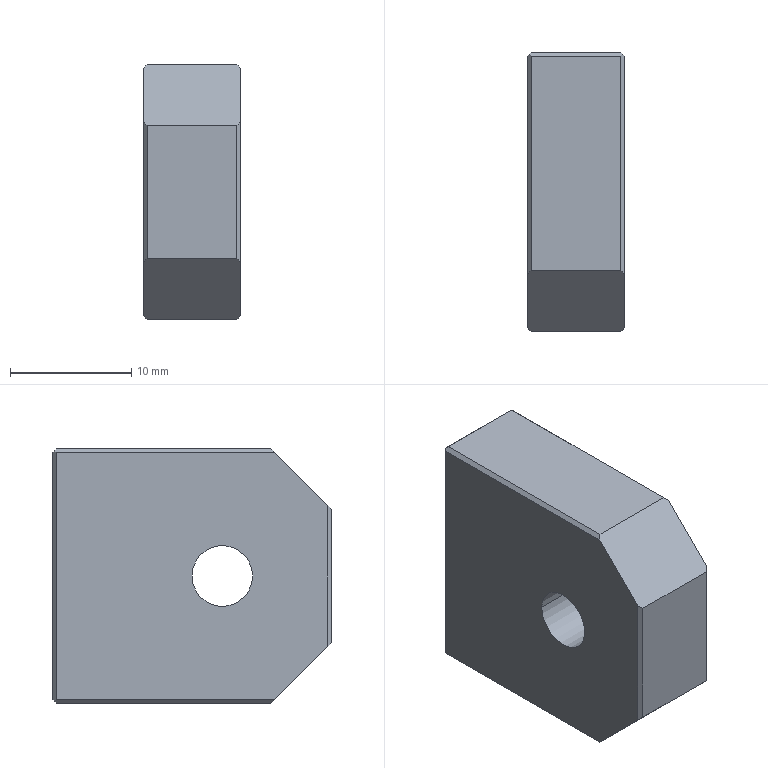Part | NX | 1 solid | 38 faces | box 8 x 23 x 21 mm | volume 3278 mm3 | plane 18 | cylinder 10 | cone 10 | commonest cylinder face diameters 3.3 x8 5 x2
STEP:
#1=CARTESIAN_POINT('',(-167.3,281.,-24.329));
#2=VERTEX_POINT('',#1);
#3=CARTESIAN_POINT('',(-174.7,281.,-24.329));
#4=VERTEX_POINT('',#3);
#5=CARTESIAN_POINT('',(-171.,281.,-24.329));
#6=DIRECTION('',(-1.,0.,0.));
#7=VECTOR('',#6,1000.);
#8=LINE('',#5,#7);
#9=EDGE_CURVE('',#2,#4,#8,.T.);
#10=ORIENTED_EDGE('',*,*,#9,.F.);
#11=CARTESIAN_POINT('',(-167.3,281.,-44.729));
#12=VERTEX_POINT('',#11);
#13=CARTESIAN_POINT('',(-167.3,281.,-34.529));
#14=DIRECTION('',(0.,0.,1.));
#15=VECTOR('',#14,1000.);
#16=LINE('',#13,#15);
#17=EDGE_CURVE('',#12,#2,#16,.T.);
#18=ORIENTED_EDGE('',*,*,#17,.F.);
#19=CARTESIAN_POINT('',(-174.7,281.,-44.729));
#20=VERTEX_POINT('',#19);
#21=CARTESIAN_POINT('',(-171.,281.,-44.729));
#22=DIRECTION('',(1.,0.,0.));
#23=VECTOR('',#22,1000.);
#24=LINE('',#21,#23);
#25=EDGE_CURVE('',#20,#12,#24,.T.);
#26=ORIENTED_EDGE('',*,*,#25,.F.);
#27=CARTESIAN_POINT('',(-174.7,281.,-34.529));
#28=DIRECTION('',(0.,0.,1.));
#29=VECTOR('',#28,1000.);
#30=LINE('',#27,#29);
#31=EDGE_CURVE('',#20,#4,#30,.T.);
#32=ORIENTED_EDGE('',*,*,#31,.T.);
#33=EDGE_LOOP('',(#10,#18,#26,#32));
#34=FACE_BOUND('',#33,.T.);
#35=CARTESIAN_POINT('',(-171.,281.,-37.464));
#36=VERTEX_POINT('',#35);
#37=CARTESIAN_POINT('',(-171.,281.,-42.094));
#38=VERTEX_POINT('',#37);
#39=CARTESIAN_POINT('',(-171.,281.,-39.779));
#40=DIRECTION('',(0.,1.,0.));
#41=DIRECTION('',(0.,0.,-1.));
#42=AXIS2_PLACEMENT_3D('',#39,#40,#41);
#43=CIRCLE('',#42,2.315);
#44=EDGE_CURVE('',#36,#38,#43,.T.);
#45=ORIENTED_EDGE('',*,*,#44,.F.);
#46=CARTESIAN_POINT('',(-171.,281.,-39.779));
#47=DIRECTION('',(0.,1.,0.));
#48=DIRECTION('',(0.,0.,-1.));
#49=AXIS2_PLACEMENT_3D('',#46,#47,#48);
#50=CIRCLE('',#49,2.315);
#51=EDGE_CURVE('',#38,#36,#50,.T.);
#52=ORIENTED_EDGE('',*,*,#51,.F.);
#53=EDGE_LOOP('',(#45,#52));
#54=FACE_BOUND('',#53,.T.);
#55=CARTESIAN_POINT('',(-171.,281.,-27.328));
#56=VERTEX_POINT('',#55);
#57=CARTESIAN_POINT('',(-171.,281.,-31.958));
#58=VERTEX_POINT('',#57);
#59=CARTESIAN_POINT('',(-171.,281.,-29.643));
#60=DIRECTION('',(0.,1.,0.));
#61=DIRECTION('',(0.,0.,-1.));
#62=AXIS2_PLACEMENT_3D('',#59,#60,#61);
#63=CIRCLE('',#62,2.315);
#64=EDGE_CURVE('',#56,#58,#63,.T.);
#65=ORIENTED_EDGE('',*,*,#64,.F.);
#66=CARTESIAN_POINT('',(-171.,281.,-29.643));
#67=DIRECTION('',(0.,1.,0.));
#68=DIRECTION('',(0.,0.,-1.));
#69=AXIS2_PLACEMENT_3D('',#66,#67,#68);
#70=CIRCLE('',#69,2.315);
#71=EDGE_CURVE('',#58,#56,#70,.T.);
#72=ORIENTED_EDGE('',*,*,#71,.F.);
#73=EDGE_LOOP('',(#65,#72));
#74=FACE_BOUND('',#73,.T.);
#75=CARTESIAN_POINT('',(-167.,281.,-45.029));
#76=DIRECTION('',(0.,1.,0.));
#77=DIRECTION('',(1.,0.,0.));
#78=AXIS2_PLACEMENT_3D('',#75,#76,#77);
#79=PLANE('',#78);
#80=ADVANCED_FACE('',(#34,#54,#74),#79,.T.);
#81=CARTESIAN_POINT('',(-167.3,263.,-45.029));
#82=VERTEX_POINT('',#81);
#83=CARTESIAN_POINT('',(-174.7,263.,-45.029));
#84=VERTEX_POINT('',#83);
#85=CARTESIAN_POINT('',(-171.,263.,-45.029));
#86=DIRECTION('',(-1.,0.,0.));
#87=VECTOR('',#86,1000.);
#88=LINE('',#85,#87);
#89=EDGE_CURVE('',#82,#84,#88,.T.);
#90=ORIENTED_EDGE('',*,*,#89,.T.);
#91=CARTESIAN_POINT('',(-174.7,280.7,-45.029));
#92=VERTEX_POINT('',#91);
#93=CARTESIAN_POINT('',(-174.7,272.,-45.029));
#94=DIRECTION('',(0.,1.,0.));
#95=VECTOR('',#94,1000.);
#96=LINE('',#93,#95);
#97=EDGE_CURVE('',#84,#92,#96,.T.);
#98=ORIENTED_EDGE('',*,*,#97,.T.);
#99=CARTESIAN_POINT('',(-167.3,280.7,-45.029));
#100=VERTEX_POINT('',#99);
#101=CARTESIAN_POINT('',(-171.,280.7,-45.029));
#102=DIRECTION('',(1.,0.,0.));
#103=VECTOR('',#102,1000.);
#104=LINE('',#101,#103);
#105=EDGE_CURVE('',#92,#100,#104,.T.);
#106=ORIENTED_EDGE('',*,*,#105,.T.);
#107=CARTESIAN_POINT('',(-167.3,272.,-45.029));
#108=DIRECTION('',(0.,1.,0.));
#109=VECTOR('',#108,1000.);
#110=LINE('',#107,#109);
#111=EDGE_CURVE('',#82,#100,#110,.T.);
#112=ORIENTED_EDGE('',*,*,#111,.F.);
#113=EDGE_LOOP('',(#90,#98,#106,#112));
#114=FACE_BOUND('',#113,.T.);
#115=CARTESIAN_POINT('',(-167.,253.,-45.029));
#116=DIRECTION('',(0.,0.,-1.));
#117=DIRECTION('',(0.,-1.,0.));
#118=AXIS2_PLACEMENT_3D('',#115,#116,#117);
#119=PLANE('',#118);
#120=ADVANCED_FACE('',(#114),#119,.T.);
#121=CARTESIAN_POINT('',(-174.7,258.,-29.029));
#122=VERTEX_POINT('',#121);
#123=CARTESIAN_POINT('',(-167.3,258.,-29.029));
#124=VERTEX_POINT('',#123);
#125=CARTESIAN_POINT('',(-171.,258.,-29.029));
#126=DIRECTION('',(1.,0.,0.));
#127=VECTOR('',#126,1000.);
#128=LINE('',#125,#127);
#129=EDGE_CURVE('',#122,#124,#128,.T.);
#130=ORIENTED_EDGE('',*,*,#129,.F.);
#131=CARTESIAN_POINT('',(-174.7,258.,-40.029));
#132=VERTEX_POINT('',#131);
#133=CARTESIAN_POINT('',(-174.7,258.,-34.529));
#134=DIRECTION('',(0.,0.,-1.));
#135=VECTOR('',#134,1000.);
#136=LINE('',#133,#135);
#137=EDGE_CURVE('',#122,#132,#136,.T.);
#138=ORIENTED_EDGE('',*,*,#137,.T.);
#139=CARTESIAN_POINT('',(-167.3,258.,-40.029));
#140=VERTEX_POINT('',#139);
#141=CARTESIAN_POINT('',(-171.,258.,-40.029));
#142=DIRECTION('',(-1.,0.,0.));
#143=VECTOR('',#142,1000.);
#144=LINE('',#141,#143);
#145=EDGE_CURVE('',#140,#132,#144,.T.);
#146=ORIENTED_EDGE('',*,*,#145,.F.);
#147=CARTESIAN_POINT('',(-167.3,258.,-34.529));
#148=DIRECTION('',(0.,0.,-1.));
#149=VECTOR('',#148,1000.);
#150=LINE('',#147,#149);
#151=EDGE_CURVE('',#124,#140,#150,.T.);
#152=ORIENTED_EDGE('',*,*,#151,.F.);
#153=EDGE_LOOP('',(#130,#138,#146,#152));
#154=FACE_BOUND('',#153,.T.);
#155=CARTESIAN_POINT('',(-167.,258.,-24.029));
#156=DIRECTION('',(0.,-1.,0.));
#157=DIRECTION('',(0.,0.,-1.));
#158=AXIS2_PLACEMENT_3D('',#155,#156,#157);
#159=PLANE('',#158);
#160=ADVANCED_FACE('',(#154),#159,.T.);
#161=CARTESIAN_POINT('',(-167.3,280.7,-24.029));
#162=VERTEX_POINT('',#161);
#163=CARTESIAN_POINT('',(-167.3,263.,-24.029));
#164=VERTEX_POINT('',#163);
#165=CARTESIAN_POINT('',(-167.3,272.,-24.029));
#166=DIRECTION('',(0.,-1.,0.));
#167=VECTOR('',#166,1000.);
#168=LINE('',#165,#167);
#169=EDGE_CURVE('',#162,#164,#168,.T.);
#170=ORIENTED_EDGE('',*,*,#169,.F.);
#171=CARTESIAN_POINT('',(-174.7,280.7,-24.029));
#172=VERTEX_POINT('',#171);
#173=CARTESIAN_POINT('',(-171.,280.7,-24.029));
#174=DIRECTION('',(-1.,0.,0.));
#175=VECTOR('',#174,1000.);
#176=LINE('',#173,#175);
#177=EDGE_CURVE('',#162,#172,#176,.T.);
#178=ORIENTED_EDGE('',*,*,#177,.T.);
#179=CARTESIAN_POINT('',(-174.7,263.,-24.029));
#180=VERTEX_POINT('',#179);
#181=CARTESIAN_POINT('',(-174.7,272.,-24.029));
#182=DIRECTION('',(0.,-1.,0.));
#183=VECTOR('',#182,1000.);
#184=LINE('',#181,#183);
#185=EDGE_CURVE('',#172,#180,#184,.T.);
#186=ORIENTED_EDGE('',*,*,#185,.T.);
#187=CARTESIAN_POINT('',(-171.,263.,-24.029));
#188=DIRECTION('',(1.,0.,0.));
#189=VECTOR('',#188,1000.);
#190=LINE('',#187,#189);
#191=EDGE_CURVE('',#180,#164,#190,.T.);
#192=ORIENTED_EDGE('',*,*,#191,.T.);
#193=EDGE_LOOP('',(#170,#178,#186,#192));
#194=FACE_BOUND('',#193,.T.);
#195=CARTESIAN_POINT('',(-167.,280.,-24.029));
#196=DIRECTION('',(0.,0.,1.));
#197=DIRECTION('',(1.,0.,0.));
#198=AXIS2_PLACEMENT_3D('',#195,#196,#197);
#199=PLANE('',#198);
#200=ADVANCED_FACE('',(#194),#199,.T.);
#201=CARTESIAN_POINT('',(-171.,280.616,-27.993));
#202=VERTEX_POINT('',#201);
#203=CARTESIAN_POINT('',(-171.,280.616,-31.293));
#204=VERTEX_POINT('',#203);
#205=CARTESIAN_POINT('',(-171.,280.616,-29.643));
#206=DIRECTION('',(0.,1.,0.));
#207=DIRECTION('',(0.,0.,-1.));
#208=AXIS2_PLACEMENT_3D('',#205,#206,#207);
#209=CIRCLE('',#208,1.65);
#210=EDGE_CURVE('',#202,#204,#209,.T.);
#211=ORIENTED_EDGE('',*,*,#210,.T.);
#212=CARTESIAN_POINT('',(-171.,273.,-31.293));
#213=VERTEX_POINT('',#212);
#214=CARTESIAN_POINT('',(-171.,281.,-31.293));
#215=DIRECTION('',(0.,1.,0.));
#216=VECTOR('',#215,1000.);
#217=LINE('',#214,#216);
#218=EDGE_CURVE('',#204,#213,#217,.F.);
#219=ORIENTED_EDGE('',*,*,#218,.T.);
#220=CARTESIAN_POINT('',(-171.,273.,-27.993));
#221=VERTEX_POINT('',#220);
#222=CARTESIAN_POINT('',(-171.,273.,-29.643));
#223=DIRECTION('',(0.,1.,0.));
#224=DIRECTION('',(0.,0.,-1.));
#225=AXIS2_PLACEMENT_3D('',#222,#223,#224);
#226=CIRCLE('',#225,1.65);
#227=EDGE_CURVE('',#221,#213,#226,.T.);
#228=ORIENTED_EDGE('',*,*,#227,.F.);
#229=CARTESIAN_POINT('',(-171.,281.,-27.993));
#230=DIRECTION('',(0.,1.,0.));
#231=VECTOR('',#230,1000.);
#232=LINE('',#229,#231);
#233=EDGE_CURVE('',#202,#221,#232,.F.);
#234=ORIENTED_EDGE('',*,*,#233,.F.);
#235=EDGE_LOOP('',(#211,#219,#228,#234));
#236=FACE_BOUND('',#235,.T.);
#237=CARTESIAN_POINT('',(-171.,281.,-29.643));
#238=DIRECTION('',(0.,1.,0.));
#239=DIRECTION('',(0.,0.,-1.));
#240=AXIS2_PLACEMENT_3D('',#237,#238,#239);
#241=CYLINDRICAL_SURFACE('',#240,1.65);
#242=ADVANCED_FACE('',(#236),#241,.F.);
#243=ORIENTED_EDGE('',*,*,#227,.T.);
#244=CARTESIAN_POINT('',(-171.,268.8,-31.293));
#245=VERTEX_POINT('',#244);
#246=CARTESIAN_POINT('',(-171.,281.,-31.293));
#247=DIRECTION('',(0.,1.,0.));
#248=VECTOR('',#247,1000.);
#249=LINE('',#246,#248);
#250=EDGE_CURVE('',#213,#245,#249,.F.);
#251=ORIENTED_EDGE('',*,*,#250,.T.);
#252=CARTESIAN_POINT('',(-171.,268.8,-27.993));
#253=VERTEX_POINT('',#252);
#254=CARTESIAN_POINT('',(-171.,268.8,-29.643));
#255=DIRECTION('',(0.,1.,0.));
#256=DIRECTION('',(0.,0.,-1.));
#257=AXIS2_PLACEMENT_3D('',#254,#255,#256);
#258=CIRCLE('',#257,1.65);
#259=EDGE_CURVE('',#253,#245,#258,.T.);
#260=ORIENTED_EDGE('',*,*,#259,.F.);
#261=CARTESIAN_POINT('',(-171.,281.,-27.993));
#262=DIRECTION('',(0.,1.,0.));
#263=VECTOR('',#262,1000.);
#264=LINE('',#261,#263);
#265=EDGE_CURVE('',#221,#253,#264,.F.);
#266=ORIENTED_EDGE('',*,*,#265,.F.);
#267=EDGE_LOOP('',(#243,#251,#260,#266));
#268=FACE_BOUND('',#267,.T.);
#269=CARTESIAN_POINT('',(-171.,281.,-29.643));
#270=DIRECTION('',(0.,1.,0.));
#271=DIRECTION('',(0.,0.,-1.));
#272=AXIS2_PLACEMENT_3D('',#269,#270,#271);
#273=CYLINDRICAL_SURFACE('',#272,1.65);
#274=ADVANCED_FACE('',(#268),#273,.F.);
#275=ORIENTED_EDGE('',*,*,#259,.T.);
#276=CARTESIAN_POINT('',(-171.,267.809,-29.643));
#277=VERTEX_POINT('',#276);
#278=CARTESIAN_POINT('',(-171.,268.8,-31.293));
#279=DIRECTION('',(0.,0.515,-0.8572));
#280=VECTOR('',#279,1000.);
#281=LINE('',#278,#280);
#282=EDGE_CURVE('',#277,#245,#281,.T.);
#283=ORIENTED_EDGE('',*,*,#282,.F.);
#284=CARTESIAN_POINT('',(-171.,268.8,-27.993));
#285=DIRECTION('',(0.,0.515,0.8572));
#286=VECTOR('',#285,1000.);
#287=LINE('',#284,#286);
#288=EDGE_CURVE('',#277,#253,#287,.T.);
#289=ORIENTED_EDGE('',*,*,#288,.T.);
#290=EDGE_LOOP('',(#275,#283,#289));
#291=FACE_BOUND('',#290,.T.);
#292=CARTESIAN_POINT('',(-171.,268.8,-29.643));
#293=DIRECTION('',(0.,1.,0.));
#294=DIRECTION('',(0.,0.,-1.));
#295=AXIS2_PLACEMENT_3D('',#292,#293,#294);
#296=CONICAL_SURFACE('',#295,1.65,1.03);
#297=ADVANCED_FACE('',(#291),#296,.F.);
#298=ORIENTED_EDGE('',*,*,#210,.F.);
#299=CARTESIAN_POINT('',(-171.,280.616,-27.993));
#300=DIRECTION('',(0.,0.5,0.866));
#301=VECTOR('',#300,1000.);
#302=LINE('',#299,#301);
#303=EDGE_CURVE('',#56,#202,#302,.F.);
#304=ORIENTED_EDGE('',*,*,#303,.F.);
#305=ORIENTED_EDGE('',*,*,#64,.T.);
#306=CARTESIAN_POINT('',(-171.,280.616,-31.293));
#307=DIRECTION('',(0.,0.5,-0.866));
#308=VECTOR('',#307,1000.);
#309=LINE('',#306,#308);
#310=EDGE_CURVE('',#58,#204,#309,.F.);
#311=ORIENTED_EDGE('',*,*,#310,.T.);
#312=EDGE_LOOP('',(#298,#304,#305,#311));
#313=FACE_BOUND('',#312,.T.);
#314=CARTESIAN_POINT('',(-171.,280.616,-29.643));
#315=DIRECTION('',(0.,1.,0.));
#316=DIRECTION('',(0.,0.,-1.));
#317=AXIS2_PLACEMENT_3D('',#314,#315,#316);
#318=CONICAL_SURFACE('',#317,1.65,1.047);
#319=ADVANCED_FACE('',(#313),#318,.F.);
#320=CARTESIAN_POINT('',(-171.,280.616,-38.129));
#321=VERTEX_POINT('',#320);
#322=CARTESIAN_POINT('',(-171.,280.616,-41.429));
#323=VERTEX_POINT('',#322);
#324=CARTESIAN_POINT('',(-171.,280.616,-39.779));
#325=DIRECTION('',(0.,1.,0.));
#326=DIRECTION('',(0.,0.,-1.));
#327=AXIS2_PLACEMENT_3D('',#324,#325,#326);
#328=CIRCLE('',#327,1.65);
#329=EDGE_CURVE('',#321,#323,#328,.T.);
#330=ORIENTED_EDGE('',*,*,#329,.T.);
#331=CARTESIAN_POINT('',(-171.,273.,-41.429));
#332=VERTEX_POINT('',#331);
#333=CARTESIAN_POINT('',(-171.,281.,-41.429));
#334=DIRECTION('',(0.,1.,0.));
#335=VECTOR('',#334,1000.);
#336=LINE('',#333,#335);
#337=EDGE_CURVE('',#323,#332,#336,.F.);
#338=ORIENTED_EDGE('',*,*,#337,.T.);
#339=CARTESIAN_POINT('',(-171.,273.,-38.129));
#340=VERTEX_POINT('',#339);
#341=CARTESIAN_POINT('',(-171.,273.,-39.779));
#342=DIRECTION('',(0.,1.,0.));
#343=DIRECTION('',(0.,0.,-1.));
#344=AXIS2_PLACEMENT_3D('',#341,#342,#343);
#345=CIRCLE('',#344,1.65);
#346=EDGE_CURVE('',#340,#332,#345,.T.);
#347=ORIENTED_EDGE('',*,*,#346,.F.);
#348=CARTESIAN_POINT('',(-171.,281.,-38.129));
#349=DIRECTION('',(0.,1.,0.));
#350=VECTOR('',#349,1000.);
#351=LINE('',#348,#350);
#352=EDGE_CURVE('',#321,#340,#351,.F.);
#353=ORIENTED_EDGE('',*,*,#352,.F.);
#354=EDGE_LOOP('',(#330,#338,#347,#353));
#355=FACE_BOUND('',#354,.T.);
#356=CARTESIAN_POINT('',(-171.,281.,-39.779));
#357=DIRECTION('',(0.,1.,0.));
#358=DIRECTION('',(0.,0.,-1.));
#359=AXIS2_PLACEMENT_3D('',#356,#357,#358);
#360=CYLINDRICAL_SURFACE('',#359,1.65);
#361=ADVANCED_FACE('',(#355),#360,.F.);
#362=ORIENTED_EDGE('',*,*,#346,.T.);
#363=CARTESIAN_POINT('',(-171.,268.8,-41.429));
#364=VERTEX_POINT('',#363);
#365=CARTESIAN_POINT('',(-171.,281.,-41.429));
#366=DIRECTION('',(0.,1.,0.));
#367=VECTOR('',#366,1000.);
#368=LINE('',#365,#367);
#369=EDGE_CURVE('',#332,#364,#368,.F.);
#370=ORIENTED_EDGE('',*,*,#369,.T.);
#371=CARTESIAN_POINT('',(-171.,268.8,-38.129));
#372=VERTEX_POINT('',#371);
#373=CARTESIAN_POINT('',(-171.,268.8,-39.779));
#374=DIRECTION('',(0.,1.,0.));
#375=DIRECTION('',(0.,0.,-1.));
#376=AXIS2_PLACEMENT_3D('',#373,#374,#375);
#377=CIRCLE('',#376,1.65);
#378=EDGE_CURVE('',#372,#364,#377,.T.);
#379=ORIENTED_EDGE('',*,*,#378,.F.);
#380=CARTESIAN_POINT('',(-171.,281.,-38.129));
#381=DIRECTION('',(0.,1.,0.));
#382=VECTOR('',#381,1000.);
#383=LINE('',#380,#382);
#384=EDGE_CURVE('',#340,#372,#383,.F.);
#385=ORIENTED_EDGE('',*,*,#384,.F.);
#386=EDGE_LOOP('',(#362,#370,#379,#385));
#387=FACE_BOUND('',#386,.T.);
#388=CARTESIAN_POINT('',(-171.,281.,-39.779));
#389=DIRECTION('',(0.,1.,0.));
#390=DIRECTION('',(0.,0.,-1.));
#391=AXIS2_PLACEMENT_3D('',#388,#389,#390);
#392=CYLINDRICAL_SURFACE('',#391,1.65);
#393=ADVANCED_FACE('',(#387),#392,.F.);
#394=ORIENTED_EDGE('',*,*,#378,.T.);
#395=CARTESIAN_POINT('',(-171.,267.809,-39.779));
#396=VERTEX_POINT('',#395);
#397=CARTESIAN_POINT('',(-171.,268.8,-41.429));
#398=DIRECTION('',(0.,0.515,-0.8572));
#399=VECTOR('',#398,1000.);
#400=LINE('',#397,#399);
#401=EDGE_CURVE('',#396,#364,#400,.T.);
#402=ORIENTED_EDGE('',*,*,#401,.F.);
#403=CARTESIAN_POINT('',(-171.,268.8,-38.129));
#404=DIRECTION('',(0.,0.515,0.8572));
#405=VECTOR('',#404,1000.);
#406=LINE('',#403,#405);
#407=EDGE_CURVE('',#396,#372,#406,.T.);
#408=ORIENTED_EDGE('',*,*,#407,.T.);
#409=EDGE_LOOP('',(#394,#402,#408));
#410=FACE_BOUND('',#409,.T.);
#411=CARTESIAN_POINT('',(-171.,268.8,-39.779));
#412=DIRECTION('',(0.,1.,0.));
#413=DIRECTION('',(0.,0.,-1.));
#414=AXIS2_PLACEMENT_3D('',#411,#412,#413);
#415=CONICAL_SURFACE('',#414,1.65,1.03);
#416=ADVANCED_FACE('',(#410),#415,.F.);
#417=ORIENTED_EDGE('',*,*,#329,.F.);
#418=CARTESIAN_POINT('',(-171.,280.616,-38.129));
#419=DIRECTION('',(0.,0.5,0.866));
#420=VECTOR('',#419,1000.);
#421=LINE('',#418,#420);
#422=EDGE_CURVE('',#36,#321,#421,.F.);
#423=ORIENTED_EDGE('',*,*,#422,.F.);
#424=ORIENTED_EDGE('',*,*,#44,.T.);
#425=CARTESIAN_POINT('',(-171.,280.616,-41.429));
#426=DIRECTION('',(0.,0.5,-0.866));
#427=VECTOR('',#426,1000.);
#428=LINE('',#425,#427);
#429=EDGE_CURVE('',#38,#323,#428,.F.);
#430=ORIENTED_EDGE('',*,*,#429,.T.);
#431=EDGE_LOOP('',(#417,#423,#424,#430));
#432=FACE_BOUND('',#431,.T.);
#433=CARTESIAN_POINT('',(-171.,280.616,-39.779));
#434=DIRECTION('',(0.,1.,0.));
#435=DIRECTION('',(0.,0.,-1.));
#436=AXIS2_PLACEMENT_3D('',#433,#434,#435);
#437=CONICAL_SURFACE('',#436,1.65,1.047);
#438=ADVANCED_FACE('',(#432),#437,.F.);
#439=ORIENTED_EDGE('',*,*,#129,.T.);
#440=CARTESIAN_POINT('',(-167.,258.3,-28.729));
#441=VERTEX_POINT('',#440);
#442=CARTESIAN_POINT('',(-170.595,254.705,-32.325));
#443=DIRECTION('',(0.5774,0.5774,0.5774));
#444=VECTOR('',#443,1000.);
#445=LINE('',#442,#444);
#446=EDGE_CURVE('',#124,#441,#445,.T.);
#447=ORIENTED_EDGE('',*,*,#446,.T.);
#448=CARTESIAN_POINT('',(-167.,262.7,-24.329));
#449=VERTEX_POINT('',#448);
#450=CARTESIAN_POINT('',(-167.,254.705,-32.325));
#451=DIRECTION('',(0.,-0.7071,-0.7071));
#452=VECTOR('',#451,1000.);
#453=LINE('',#450,#452);
#454=EDGE_CURVE('',#449,#441,#453,.T.);
#455=ORIENTED_EDGE('',*,*,#454,.F.);
#456=CARTESIAN_POINT('',(-167.,262.7,-24.329));
#457=DIRECTION('',(-0.5774,0.5774,0.5774));
#458=VECTOR('',#457,1000.);
#459=LINE('',#456,#458);
#460=EDGE_CURVE('',#449,#164,#459,.T.);
#461=ORIENTED_EDGE('',*,*,#460,.T.);
#462=ORIENTED_EDGE('',*,*,#191,.F.);
#463=CARTESIAN_POINT('',(-175.,262.7,-24.329));
#464=VERTEX_POINT('',#463);
#465=CARTESIAN_POINT('',(-167.,270.7,-16.329));
#466=DIRECTION('',(0.5774,0.5774,0.5774));
#467=VECTOR('',#466,1000.);
#468=LINE('',#465,#467);
#469=EDGE_CURVE('',#464,#180,#468,.T.);
#470=ORIENTED_EDGE('',*,*,#469,.F.);
#471=CARTESIAN_POINT('',(-175.,258.3,-28.729));
#472=VERTEX_POINT('',#471);
#473=CARTESIAN_POINT('',(-175.,254.705,-32.325));
#474=DIRECTION('',(0.,-0.7071,-0.7071));
#475=VECTOR('',#474,1000.);
#476=LINE('',#473,#475);
#477=EDGE_CURVE('',#464,#472,#476,.T.);
#478=ORIENTED_EDGE('',*,*,#477,.T.);
#479=CARTESIAN_POINT('',(-171.405,254.705,-32.325));
#480=DIRECTION('',(-0.5774,0.5774,0.5774));
#481=VECTOR('',#480,1000.);
#482=LINE('',#479,#481);
#483=EDGE_CURVE('',#122,#472,#482,.T.);
#484=ORIENTED_EDGE('',*,*,#483,.F.);
#485=EDGE_LOOP('',(#439,#447,#455,#461,#462,#470,#478,#484));
#486=FACE_BOUND('',#485,.T.);
#487=CARTESIAN_POINT('',(-171.,260.5,-26.529));
#488=DIRECTION('',(0.,0.7071,-0.7071));
#489=DIRECTION('',(-1.,0.,0.));
#490=AXIS2_PLACEMENT_3D('',#487,#488,#489);
#491=PLANE('',#490);
#492=ADVANCED_FACE('',(#486),#491,.F.);
#493=ORIENTED_EDGE('',*,*,#89,.F.);
#494=CARTESIAN_POINT('',(-167.,262.7,-44.729));
#495=VERTEX_POINT('',#494);
#496=CARTESIAN_POINT('',(-154.595,250.295,-32.325));
#497=DIRECTION('',(-0.5774,0.5774,-0.5774));
#498=VECTOR('',#497,1000.);
#499=LINE('',#496,#498);
#500=EDGE_CURVE('',#495,#82,#499,.T.);
#501=ORIENTED_EDGE('',*,*,#500,.F.);
#502=CARTESIAN_POINT('',(-167.,258.3,-40.329));
#503=VERTEX_POINT('',#502);
#504=CARTESIAN_POINT('',(-167.,250.295,-32.325));
#505=DIRECTION('',(0.,-0.7071,0.7071));
#506=VECTOR('',#505,1000.);
#507=LINE('',#504,#506);
#508=EDGE_CURVE('',#495,#503,#507,.T.);
#509=ORIENTED_EDGE('',*,*,#508,.T.);
#510=CARTESIAN_POINT('',(-175.005,250.295,-32.325));
#511=DIRECTION('',(0.5774,0.5774,-0.5774));
#512=VECTOR('',#511,1000.);
#513=LINE('',#510,#512);
#514=EDGE_CURVE('',#140,#503,#513,.T.);
#515=ORIENTED_EDGE('',*,*,#514,.F.);
#516=ORIENTED_EDGE('',*,*,#145,.T.);
#517=CARTESIAN_POINT('',(-175.,258.3,-40.329));
#518=VERTEX_POINT('',#517);
#519=CARTESIAN_POINT('',(-166.995,250.295,-32.325));
#520=DIRECTION('',(-0.5774,0.5774,-0.5774));
#521=VECTOR('',#520,1000.);
#522=LINE('',#519,#521);
#523=EDGE_CURVE('',#132,#518,#522,.T.);
#524=ORIENTED_EDGE('',*,*,#523,.T.);
#525=CARTESIAN_POINT('',(-175.,262.7,-44.729));
#526=VERTEX_POINT('',#525);
#527=CARTESIAN_POINT('',(-175.,250.295,-32.325));
#528=DIRECTION('',(0.,-0.7071,0.7071));
#529=VECTOR('',#528,1000.);
#530=LINE('',#527,#529);
#531=EDGE_CURVE('',#526,#518,#530,.T.);
#532=ORIENTED_EDGE('',*,*,#531,.F.);
#533=CARTESIAN_POINT('',(-187.405,250.295,-32.325));
#534=DIRECTION('',(0.5774,0.5774,-0.5774));
#535=VECTOR('',#534,1000.);
#536=LINE('',#533,#535);
#537=EDGE_CURVE('',#526,#84,#536,.T.);
#538=ORIENTED_EDGE('',*,*,#537,.T.);
#539=EDGE_LOOP('',(#493,#501,#509,#515,#516,#524,#532,#538));
#540=FACE_BOUND('',#539,.T.);
#541=CARTESIAN_POINT('',(-171.,260.5,-42.529));
#542=DIRECTION('',(0.,-0.7071,-0.7071));
#543=DIRECTION('',(0.,-0.7071,0.7071));
#544=AXIS2_PLACEMENT_3D('',#541,#542,#543);
#545=PLANE('',#544);
#546=ADVANCED_FACE('',(#540),#545,.T.);
#547=ORIENTED_EDGE('',*,*,#25,.T.);
#548=CARTESIAN_POINT('',(-167.15,280.85,-44.879));
#549=VERTEX_POINT('',#548);
#550=CARTESIAN_POINT('',(-167.,280.7,-45.029));
#551=DIRECTION('',(0.5774,-0.5774,-0.5774));
#552=VECTOR('',#551,1000.);
#553=LINE('',#550,#552);
#554=EDGE_CURVE('',#12,#549,#553,.T.);
#555=ORIENTED_EDGE('',*,*,#554,.T.);
#556=CARTESIAN_POINT('',(-154.595,293.405,-32.325));
#557=DIRECTION('',(0.5774,0.5774,0.5774));
#558=VECTOR('',#557,1000.);
#559=LINE('',#556,#558);
#560=EDGE_CURVE('',#100,#549,#559,.T.);
#561=ORIENTED_EDGE('',*,*,#560,.F.);
#562=ORIENTED_EDGE('',*,*,#105,.F.);
#563=CARTESIAN_POINT('',(-174.85,280.85,-44.879));
#564=VERTEX_POINT('',#563);
#565=CARTESIAN_POINT('',(-187.405,293.405,-32.325));
#566=DIRECTION('',(-0.5774,0.5774,0.5774));
#567=VECTOR('',#566,1000.);
#568=LINE('',#565,#567);
#569=EDGE_CURVE('',#92,#564,#568,.T.);
#570=ORIENTED_EDGE('',*,*,#569,.T.);
#571=CARTESIAN_POINT('',(-167.,288.7,-37.029));
#572=DIRECTION('',(0.5774,0.5774,0.5774));
#573=VECTOR('',#572,1000.);
#574=LINE('',#571,#573);
#575=EDGE_CURVE('',#564,#20,#574,.T.);
#576=ORIENTED_EDGE('',*,*,#575,.T.);
#577=EDGE_LOOP('',(#547,#555,#561,#562,#570,#576));
#578=FACE_BOUND('',#577,.T.);
#579=CARTESIAN_POINT('',(-171.,280.85,-44.879));
#580=DIRECTION('',(0.,-0.7071,0.7071));
#581=DIRECTION('',(-1.,0.,0.));
#582=AXIS2_PLACEMENT_3D('',#579,#580,#581);
#583=PLANE('',#582);
#584=ADVANCED_FACE('',(#578),#583,.F.);
#585=ORIENTED_EDGE('',*,*,#9,.T.);
#586=CARTESIAN_POINT('',(-174.85,280.85,-24.179));
#587=VERTEX_POINT('',#586);
#588=CARTESIAN_POINT('',(-166.705,288.995,-32.325));
#589=DIRECTION('',(0.5774,0.5774,-0.5774));
#590=VECTOR('',#589,1000.);
#591=LINE('',#588,#590);
#592=EDGE_CURVE('',#587,#4,#591,.T.);
#593=ORIENTED_EDGE('',*,*,#592,.F.);
#594=CARTESIAN_POINT('',(-167.,273.,-16.329));
#595=DIRECTION('',(0.5774,-0.5774,0.5774));
#596=VECTOR('',#595,1000.);
#597=LINE('',#594,#596);
#598=EDGE_CURVE('',#587,#172,#597,.T.);
#599=ORIENTED_EDGE('',*,*,#598,.T.);
#600=ORIENTED_EDGE('',*,*,#177,.F.);
#601=CARTESIAN_POINT('',(-167.15,280.85,-24.179));
#602=VERTEX_POINT('',#601);
#603=CARTESIAN_POINT('',(-167.,281.,-24.329));
#604=DIRECTION('',(-0.5774,-0.5774,0.5774));
#605=VECTOR('',#604,1000.);
#606=LINE('',#603,#605);
#607=EDGE_CURVE('',#602,#162,#606,.T.);
#608=ORIENTED_EDGE('',*,*,#607,.F.);
#609=CARTESIAN_POINT('',(-175.295,288.995,-32.325));
#610=DIRECTION('',(-0.5774,0.5774,-0.5774));
#611=VECTOR('',#610,1000.);
#612=LINE('',#609,#611);
#613=EDGE_CURVE('',#602,#2,#612,.T.);
#614=ORIENTED_EDGE('',*,*,#613,.T.);
#615=EDGE_LOOP('',(#585,#593,#599,#600,#608,#614));
#616=FACE_BOUND('',#615,.T.);
#617=CARTESIAN_POINT('',(-171.,280.85,-24.179));
#618=DIRECTION('',(0.,-0.7071,-0.7071));
#619=DIRECTION('',(0.,0.7071,-0.7071));
#620=AXIS2_PLACEMENT_3D('',#617,#618,#619);
#621=PLANE('',#620);
#622=ADVANCED_FACE('',(#616),#621,.F.);
#623=ORIENTED_EDGE('',*,*,#407,.F.);
#624=ORIENTED_EDGE('',*,*,#401,.T.);
#625=CARTESIAN_POINT('',(-171.,268.8,-39.779));
#626=DIRECTION('',(0.,1.,0.));
#627=DIRECTION('',(0.,0.,-1.));
#628=AXIS2_PLACEMENT_3D('',#625,#626,#627);
#629=CIRCLE('',#628,1.65);
#630=EDGE_CURVE('',#364,#372,#629,.T.);
#631=ORIENTED_EDGE('',*,*,#630,.T.);
#632=EDGE_LOOP('',(#623,#624,#631));
#633=FACE_BOUND('',#632,.T.);
#634=CARTESIAN_POINT('',(-171.,268.8,-39.779));
#635=DIRECTION('',(0.,1.,0.));
#636=DIRECTION('',(0.,0.,-1.));
#637=AXIS2_PLACEMENT_3D('',#634,#635,#636);
#638=CONICAL_SURFACE('',#637,1.65,1.03);
#639=ADVANCED_FACE('',(#633),#638,.F.);
#640=ORIENTED_EDGE('',*,*,#429,.F.);
#641=ORIENTED_EDGE('',*,*,#51,.T.);
#642=ORIENTED_EDGE('',*,*,#422,.T.);
#643=CARTESIAN_POINT('',(-171.,280.616,-39.779));
#644=DIRECTION('',(0.,1.,0.));
#645=DIRECTION('',(0.,0.,-1.));
#646=AXIS2_PLACEMENT_3D('',#643,#644,#645);
#647=CIRCLE('',#646,1.65);
#648=EDGE_CURVE('',#323,#321,#647,.T.);
#649=ORIENTED_EDGE('',*,*,#648,.F.);
#650=EDGE_LOOP('',(#640,#641,#642,#649));
#651=FACE_BOUND('',#650,.T.);
#652=CARTESIAN_POINT('',(-171.,280.616,-39.779));
#653=DIRECTION('',(0.,1.,0.));
#654=DIRECTION('',(0.,0.,-1.));
#655=AXIS2_PLACEMENT_3D('',#652,#653,#654);
#656=CONICAL_SURFACE('',#655,1.65,1.047);
#657=ADVANCED_FACE('',(#651),#656,.F.);
#658=ORIENTED_EDGE('',*,*,#250,.F.);
#659=CARTESIAN_POINT('',(-171.,273.,-29.643));
#660=DIRECTION('',(0.,1.,0.));
#661=DIRECTION('',(0.,0.,-1.));
#662=AXIS2_PLACEMENT_3D('',#659,#660,#661);
#663=CIRCLE('',#662,1.65);
#664=EDGE_CURVE('',#213,#221,#663,.T.);
#665=ORIENTED_EDGE('',*,*,#664,.T.);
#666=ORIENTED_EDGE('',*,*,#265,.T.);
#667=CARTESIAN_POINT('',(-171.,268.8,-29.643));
#668=DIRECTION('',(0.,1.,0.));
#669=DIRECTION('',(0.,0.,-1.));
#670=AXIS2_PLACEMENT_3D('',#667,#668,#669);
#671=CIRCLE('',#670,1.65);
#672=EDGE_CURVE('',#245,#253,#671,.T.);
#673=ORIENTED_EDGE('',*,*,#672,.F.);
#674=EDGE_LOOP('',(#658,#665,#666,#673));
#675=FACE_BOUND('',#674,.T.);
#676=CARTESIAN_POINT('',(-171.,281.,-29.643));
#677=DIRECTION('',(0.,1.,0.));
#678=DIRECTION('',(0.,0.,-1.));
#679=AXIS2_PLACEMENT_3D('',#676,#677,#678);
#680=CYLINDRICAL_SURFACE('',#679,1.65);
#681=ADVANCED_FACE('',(#675),#680,.F.);
#682=ORIENTED_EDGE('',*,*,#337,.F.);
#683=ORIENTED_EDGE('',*,*,#648,.T.);
#684=ORIENTED_EDGE('',*,*,#352,.T.);
#685=CARTESIAN_POINT('',(-171.,273.,-39.779));
#686=DIRECTION('',(0.,1.,0.));
#687=DIRECTION('',(0.,0.,-1.));
#688=AXIS2_PLACEMENT_3D('',#685,#686,#687);
#689=CIRCLE('',#688,1.65);
#690=EDGE_CURVE('',#332,#340,#689,.T.);
#691=ORIENTED_EDGE('',*,*,#690,.F.);
#692=EDGE_LOOP('',(#682,#683,#684,#691));
#693=FACE_BOUND('',#692,.T.);
#694=CARTESIAN_POINT('',(-171.,281.,-39.779));
#695=DIRECTION('',(0.,1.,0.));
#696=DIRECTION('',(0.,0.,-1.));
#697=AXIS2_PLACEMENT_3D('',#694,#695,#696);
#698=CYLINDRICAL_SURFACE('',#697,1.65);
#699=ADVANCED_FACE('',(#693),#698,.F.);
#700=ORIENTED_EDGE('',*,*,#288,.F.);
#701=ORIENTED_EDGE('',*,*,#282,.T.);
#702=ORIENTED_EDGE('',*,*,#672,.T.);
#703=EDGE_LOOP('',(#700,#701,#702));
#704=FACE_BOUND('',#703,.T.);
#705=CARTESIAN_POINT('',(-171.,268.8,-29.643));
#706=DIRECTION('',(0.,1.,0.));
#707=DIRECTION('',(0.,0.,-1.));
#708=AXIS2_PLACEMENT_3D('',#705,#706,#707);
#709=CONICAL_SURFACE('',#708,1.65,1.03);
#710=ADVANCED_FACE('',(#704),#709,.F.);
#711=ORIENTED_EDGE('',*,*,#310,.F.);
#712=ORIENTED_EDGE('',*,*,#71,.T.);
#713=ORIENTED_EDGE('',*,*,#303,.T.);
#714=CARTESIAN_POINT('',(-171.,280.616,-29.643));
#715=DIRECTION('',(0.,1.,0.));
#716=DIRECTION('',(0.,0.,-1.));
#717=AXIS2_PLACEMENT_3D('',#714,#715,#716);
#718=CIRCLE('',#717,1.65);
#719=EDGE_CURVE('',#204,#202,#718,.T.);
#720=ORIENTED_EDGE('',*,*,#719,.F.);
#721=EDGE_LOOP('',(#711,#712,#713,#720));
#722=FACE_BOUND('',#721,.T.);
#723=CARTESIAN_POINT('',(-171.,280.616,-29.643));
#724=DIRECTION('',(0.,1.,0.));
#725=DIRECTION('',(0.,0.,-1.));
#726=AXIS2_PLACEMENT_3D('',#723,#724,#725);
#727=CONICAL_SURFACE('',#726,1.65,1.047);
#728=ADVANCED_FACE('',(#722),#727,.F.);
#729=ORIENTED_EDGE('',*,*,#369,.F.);
#730=ORIENTED_EDGE('',*,*,#690,.T.);
#731=ORIENTED_EDGE('',*,*,#384,.T.);
#732=ORIENTED_EDGE('',*,*,#630,.F.);
#733=EDGE_LOOP('',(#729,#730,#731,#732));
#734=FACE_BOUND('',#733,.T.);
#735=CARTESIAN_POINT('',(-171.,281.,-39.779));
#736=DIRECTION('',(0.,1.,0.));
#737=DIRECTION('',(0.,0.,-1.));
#738=AXIS2_PLACEMENT_3D('',#735,#736,#737);
#739=CYLINDRICAL_SURFACE('',#738,1.65);
#740=ADVANCED_FACE('',(#734),#739,.F.);
#741=ORIENTED_EDGE('',*,*,#218,.F.);
#742=ORIENTED_EDGE('',*,*,#719,.T.);
#743=ORIENTED_EDGE('',*,*,#233,.T.);
#744=ORIENTED_EDGE('',*,*,#664,.F.);
#745=EDGE_LOOP('',(#741,#742,#743,#744));
#746=FACE_BOUND('',#745,.T.);
#747=CARTESIAN_POINT('',(-171.,281.,-29.643));
#748=DIRECTION('',(0.,1.,0.));
#749=DIRECTION('',(0.,0.,-1.));
#750=AXIS2_PLACEMENT_3D('',#747,#748,#749);
#751=CYLINDRICAL_SURFACE('',#750,1.65);
#752=ADVANCED_FACE('',(#746),#751,.F.);
#753=CARTESIAN_POINT('',(-175.,258.3,-34.529));
#754=DIRECTION('',(0.,0.,-1.));
#755=VECTOR('',#754,1000.);
#756=LINE('',#753,#755);
#757=EDGE_CURVE('',#472,#518,#756,.T.);
#758=ORIENTED_EDGE('',*,*,#757,.F.);
#759=ORIENTED_EDGE('',*,*,#477,.F.);
#760=CARTESIAN_POINT('',(-175.,280.7,-24.329));
#761=VERTEX_POINT('',#760);
#762=CARTESIAN_POINT('',(-175.,272.,-24.329));
#763=DIRECTION('',(0.,-1.,0.));
#764=VECTOR('',#763,1000.);
#765=LINE('',#762,#764);
#766=EDGE_CURVE('',#761,#464,#765,.T.);
#767=ORIENTED_EDGE('',*,*,#766,.F.);
#768=CARTESIAN_POINT('',(-175.,280.7,-44.729));
#769=VERTEX_POINT('',#768);
#770=CARTESIAN_POINT('',(-175.,280.7,-34.529));
#771=DIRECTION('',(0.,0.,1.));
#772=VECTOR('',#771,1000.);
#773=LINE('',#770,#772);
#774=EDGE_CURVE('',#769,#761,#773,.T.);
#775=ORIENTED_EDGE('',*,*,#774,.F.);
#776=CARTESIAN_POINT('',(-175.,272.,-44.729));
#777=DIRECTION('',(0.,1.,0.));
#778=VECTOR('',#777,1000.);
#779=LINE('',#776,#778);
#780=EDGE_CURVE('',#526,#769,#779,.T.);
#781=ORIENTED_EDGE('',*,*,#780,.F.);
#782=ORIENTED_EDGE('',*,*,#531,.T.);
#783=EDGE_LOOP('',(#758,#759,#767,#775,#781,#782));
#784=FACE_BOUND('',#783,.T.);
#785=CARTESIAN_POINT('',(-175.,264.5,-34.529));
#786=VERTEX_POINT('',#785);
#787=CARTESIAN_POINT('',(-175.,269.5,-34.529));
#788=VERTEX_POINT('',#787);
#789=CARTESIAN_POINT('',(-175.,267.,-34.529));
#790=DIRECTION('',(1.,0.,0.));
#791=DIRECTION('',(0.,1.,0.));
#792=AXIS2_PLACEMENT_3D('',#789,#790,#791);
#793=CIRCLE('',#792,2.5);
#794=EDGE_CURVE('',#786,#788,#793,.T.);
#795=ORIENTED_EDGE('',*,*,#794,.T.);
#796=CARTESIAN_POINT('',(-175.,267.,-34.529));
#797=DIRECTION('',(1.,0.,0.));
#798=DIRECTION('',(0.,1.,0.));
#799=AXIS2_PLACEMENT_3D('',#796,#797,#798);
#800=CIRCLE('',#799,2.5);
#801=EDGE_CURVE('',#788,#786,#800,.T.);
#802=ORIENTED_EDGE('',*,*,#801,.T.);
#803=EDGE_LOOP('',(#795,#802));
#804=FACE_BOUND('',#803,.T.);
#805=CARTESIAN_POINT('',(-175.,285.476,-32.325));
#806=DIRECTION('',(1.,0.,0.));
#807=DIRECTION('',(0.,1.,0.));
#808=AXIS2_PLACEMENT_3D('',#805,#806,#807);
#809=PLANE('',#808);
#810=ADVANCED_FACE('',(#784,#804),#809,.F.);
#811=CARTESIAN_POINT('',(-167.548,264.5,-34.529));
#812=VERTEX_POINT('',#811);
#813=CARTESIAN_POINT('',(-167.548,269.5,-34.529));
#814=VERTEX_POINT('',#813);
#815=CARTESIAN_POINT('',(-167.548,267.,-34.529));
#816=DIRECTION('',(1.,0.,0.));
#817=DIRECTION('',(0.,1.,0.));
#818=AXIS2_PLACEMENT_3D('',#815,#816,#817);
#819=CIRCLE('',#818,2.5);
#820=EDGE_CURVE('',#812,#814,#819,.T.);
#821=ORIENTED_EDGE('',*,*,#820,.T.);
#822=CARTESIAN_POINT('',(-167.,269.5,-34.529));
#823=DIRECTION('',(1.,0.,0.));
#824=VECTOR('',#823,1000.);
#825=LINE('',#822,#824);
#826=EDGE_CURVE('',#788,#814,#825,.T.);
#827=ORIENTED_EDGE('',*,*,#826,.F.);
#828=ORIENTED_EDGE('',*,*,#794,.F.);
#829=CARTESIAN_POINT('',(-167.,264.5,-34.529));
#830=DIRECTION('',(1.,0.,0.));
#831=VECTOR('',#830,1000.);
#832=LINE('',#829,#831);
#833=EDGE_CURVE('',#786,#812,#832,.T.);
#834=ORIENTED_EDGE('',*,*,#833,.T.);
#835=EDGE_LOOP('',(#821,#827,#828,#834));
#836=FACE_BOUND('',#835,.T.);
#837=CARTESIAN_POINT('',(-167.,267.,-34.529));
#838=DIRECTION('',(1.,0.,0.));
#839=DIRECTION('',(0.,1.,0.));
#840=AXIS2_PLACEMENT_3D('',#837,#838,#839);
#841=CYLINDRICAL_SURFACE('',#840,2.5);
#842=ADVANCED_FACE('',(#836),#841,.F.);
#843=ORIENTED_EDGE('',*,*,#820,.F.);
#844=CARTESIAN_POINT('',(-167.,263.55,-34.529));
#845=VERTEX_POINT('',#844);
#846=CARTESIAN_POINT('',(-167.548,264.5,-34.529));
#847=DIRECTION('',(0.5,-0.866,0.));
#848=VECTOR('',#847,1000.);
#849=LINE('',#846,#848);
#850=EDGE_CURVE('',#812,#845,#849,.T.);
#851=ORIENTED_EDGE('',*,*,#850,.T.);
#852=CARTESIAN_POINT('',(-167.,270.45,-34.529));
#853=VERTEX_POINT('',#852);
#854=CARTESIAN_POINT('',(-167.,267.,-34.529));
#855=DIRECTION('',(1.,0.,0.));
#856=DIRECTION('',(0.,1.,0.));
#857=AXIS2_PLACEMENT_3D('',#854,#855,#856);
#858=CIRCLE('',#857,3.45);
#859=EDGE_CURVE('',#845,#853,#858,.T.);
#860=ORIENTED_EDGE('',*,*,#859,.T.);
#861=CARTESIAN_POINT('',(-167.548,269.5,-34.529));
#862=DIRECTION('',(0.5,0.866,0.));
#863=VECTOR('',#862,1000.);
#864=LINE('',#861,#863);
#865=EDGE_CURVE('',#814,#853,#864,.T.);
#866=ORIENTED_EDGE('',*,*,#865,.F.);
#867=EDGE_LOOP('',(#843,#851,#860,#866));
#868=FACE_BOUND('',#867,.T.);
#869=CARTESIAN_POINT('',(-167.548,267.,-34.529));
#870=DIRECTION('',(1.,0.,0.));
#871=DIRECTION('',(0.,1.,0.));
#872=AXIS2_PLACEMENT_3D('',#869,#870,#871);
#873=CONICAL_SURFACE('',#872,2.5,1.047);
#874=ADVANCED_FACE('',(#868),#873,.F.);
#875=ORIENTED_EDGE('',*,*,#774,.T.);
#876=CARTESIAN_POINT('',(-167.,288.7,-16.329));
#877=DIRECTION('',(0.5774,0.5774,0.5774));
#878=VECTOR('',#877,1000.);
#879=LINE('',#876,#878);
#880=EDGE_CURVE('',#761,#587,#879,.T.);
#881=ORIENTED_EDGE('',*,*,#880,.T.);
#882=ORIENTED_EDGE('',*,*,#592,.T.);
#883=ORIENTED_EDGE('',*,*,#31,.F.);
#884=ORIENTED_EDGE('',*,*,#575,.F.);
#885=CARTESIAN_POINT('',(-187.405,268.295,-32.325));
#886=DIRECTION('',(-0.5774,-0.5774,0.5774));
#887=VECTOR('',#886,1000.);
#888=LINE('',#885,#887);
#889=EDGE_CURVE('',#564,#769,#888,.T.);
#890=ORIENTED_EDGE('',*,*,#889,.T.);
#891=EDGE_LOOP('',(#875,#881,#882,#883,#884,#890));
#892=FACE_BOUND('',#891,.T.);
#893=CARTESIAN_POINT('',(-174.85,280.85,-34.529));
#894=DIRECTION('',(0.7071,-0.7071,0.));
#895=DIRECTION('',(0.,0.,-1.));
#896=AXIS2_PLACEMENT_3D('',#893,#894,#895);
#897=PLANE('',#896);
#898=ADVANCED_FACE('',(#892),#897,.F.);
#899=ORIENTED_EDGE('',*,*,#766,.T.);
#900=ORIENTED_EDGE('',*,*,#469,.T.);
#901=ORIENTED_EDGE('',*,*,#185,.F.);
#902=ORIENTED_EDGE('',*,*,#598,.F.);
#903=ORIENTED_EDGE('',*,*,#880,.F.);
#904=EDGE_LOOP('',(#899,#900,#901,#902,#903));
#905=FACE_BOUND('',#904,.T.);
#906=CARTESIAN_POINT('',(-174.85,272.,-24.179));
#907=DIRECTION('',(0.7071,0.,-0.7071));
#908=DIRECTION('',(0.,-1.,0.));
#909=AXIS2_PLACEMENT_3D('',#906,#907,#908);
#910=PLANE('',#909);
#911=ADVANCED_FACE('',(#905),#910,.F.);
#912=ORIENTED_EDGE('',*,*,#780,.T.);
#913=ORIENTED_EDGE('',*,*,#889,.F.);
#914=ORIENTED_EDGE('',*,*,#569,.F.);
#915=ORIENTED_EDGE('',*,*,#97,.F.);
#916=ORIENTED_EDGE('',*,*,#537,.F.);
#917=EDGE_LOOP('',(#912,#913,#914,#915,#916));
#918=FACE_BOUND('',#917,.T.);
#919=CARTESIAN_POINT('',(-174.85,272.,-44.879));
#920=DIRECTION('',(0.7071,0.,0.7071));
#921=DIRECTION('',(0.,-1.,0.));
#922=AXIS2_PLACEMENT_3D('',#919,#920,#921);
#923=PLANE('',#922);
#924=ADVANCED_FACE('',(#918),#923,.F.);
#925=ORIENTED_EDGE('',*,*,#757,.T.);
#926=ORIENTED_EDGE('',*,*,#523,.F.);
#927=ORIENTED_EDGE('',*,*,#137,.F.);
#928=ORIENTED_EDGE('',*,*,#483,.T.);
#929=EDGE_LOOP('',(#925,#926,#927,#928));
#930=FACE_BOUND('',#929,.T.);
#931=CARTESIAN_POINT('',(-174.85,258.15,-34.529));
#932=DIRECTION('',(0.7071,0.7071,0.));
#933=DIRECTION('',(0.,0.,-1.));
#934=AXIS2_PLACEMENT_3D('',#931,#932,#933);
#935=PLANE('',#934);
#936=ADVANCED_FACE('',(#930),#935,.F.);
#937=ORIENTED_EDGE('',*,*,#865,.T.);
#938=CARTESIAN_POINT('',(-167.,267.,-34.529));
#939=DIRECTION('',(1.,0.,0.));
#940=DIRECTION('',(0.,1.,0.));
#941=AXIS2_PLACEMENT_3D('',#938,#939,#940);
#942=CIRCLE('',#941,3.45);
#943=EDGE_CURVE('',#853,#845,#942,.T.);
#944=ORIENTED_EDGE('',*,*,#943,.T.);
#945=ORIENTED_EDGE('',*,*,#850,.F.);
#946=CARTESIAN_POINT('',(-167.548,267.,-34.529));
#947=DIRECTION('',(1.,0.,0.));
#948=DIRECTION('',(0.,1.,0.));
#949=AXIS2_PLACEMENT_3D('',#946,#947,#948);
#950=CIRCLE('',#949,2.5);
#951=EDGE_CURVE('',#814,#812,#950,.T.);
#952=ORIENTED_EDGE('',*,*,#951,.F.);
#953=EDGE_LOOP('',(#937,#944,#945,#952));
#954=FACE_BOUND('',#953,.T.);
#955=CARTESIAN_POINT('',(-167.548,267.,-34.529));
#956=DIRECTION('',(1.,0.,0.));
#957=DIRECTION('',(0.,1.,0.));
#958=AXIS2_PLACEMENT_3D('',#955,#956,#957);
#959=CONICAL_SURFACE('',#958,2.5,1.047);
#960=ADVANCED_FACE('',(#954),#959,.F.);
#961=ORIENTED_EDGE('',*,*,#826,.T.);
#962=ORIENTED_EDGE('',*,*,#951,.T.);
#963=ORIENTED_EDGE('',*,*,#833,.F.);
#964=ORIENTED_EDGE('',*,*,#801,.F.);
#965=EDGE_LOOP('',(#961,#962,#963,#964));
#966=FACE_BOUND('',#965,.T.);
#967=CARTESIAN_POINT('',(-167.,267.,-34.529));
#968=DIRECTION('',(1.,0.,0.));
#969=DIRECTION('',(0.,1.,0.));
#970=AXIS2_PLACEMENT_3D('',#967,#968,#969);
#971=CYLINDRICAL_SURFACE('',#970,2.5);
#972=ADVANCED_FACE('',(#966),#971,.F.);
#973=CARTESIAN_POINT('',(-167.,258.3,-34.529));
#974=DIRECTION('',(0.,0.,-1.));
#975=VECTOR('',#974,1000.);
#976=LINE('',#973,#975);
#977=EDGE_CURVE('',#441,#503,#976,.T.);
#978=ORIENTED_EDGE('',*,*,#977,.T.);
#979=ORIENTED_EDGE('',*,*,#508,.F.);
#980=CARTESIAN_POINT('',(-167.,280.7,-44.729));
#981=VERTEX_POINT('',#980);
#982=CARTESIAN_POINT('',(-167.,272.,-44.729));
#983=DIRECTION('',(0.,1.,0.));
#984=VECTOR('',#983,1000.);
#985=LINE('',#982,#984);
#986=EDGE_CURVE('',#495,#981,#985,.T.);
#987=ORIENTED_EDGE('',*,*,#986,.T.);
#988=CARTESIAN_POINT('',(-167.,280.7,-24.329));
#989=VERTEX_POINT('',#988);
#990=CARTESIAN_POINT('',(-167.,280.7,-34.529));
#991=DIRECTION('',(0.,0.,1.));
#992=VECTOR('',#991,1000.);
#993=LINE('',#990,#992);
#994=EDGE_CURVE('',#981,#989,#993,.T.);
#995=ORIENTED_EDGE('',*,*,#994,.T.);
#996=CARTESIAN_POINT('',(-167.,272.,-24.329));
#997=DIRECTION('',(0.,-1.,0.));
#998=VECTOR('',#997,1000.);
#999=LINE('',#996,#998);
#1000=EDGE_CURVE('',#989,#449,#999,.T.);
#1001=ORIENTED_EDGE('',*,*,#1000,.T.);
#1002=ORIENTED_EDGE('',*,*,#454,.T.);
#1003=EDGE_LOOP('',(#978,#979,#987,#995,#1001,#1002));
#1004=FACE_BOUND('',#1003,.T.);
#1005=ORIENTED_EDGE('',*,*,#859,.F.);
#1006=ORIENTED_EDGE('',*,*,#943,.F.);
#1007=EDGE_LOOP('',(#1005,#1006));
#1008=FACE_BOUND('',#1007,.T.);
#1009=CARTESIAN_POINT('',(-167.,285.476,-32.325));
#1010=DIRECTION('',(1.,0.,0.));
#1011=DIRECTION('',(0.,1.,0.));
#1012=AXIS2_PLACEMENT_3D('',#1009,#1010,#1011);
#1013=PLANE('',#1012);
#1014=ADVANCED_FACE('',(#1004,#1008),#1013,.T.);
#1015=ORIENTED_EDGE('',*,*,#994,.F.);
#1016=CARTESIAN_POINT('',(-154.595,268.295,-32.325));
#1017=DIRECTION('',(-0.5774,0.5774,-0.5774));
#1018=VECTOR('',#1017,1000.);
#1019=LINE('',#1016,#1018);
#1020=EDGE_CURVE('',#981,#549,#1019,.T.);
#1021=ORIENTED_EDGE('',*,*,#1020,.T.);
#1022=ORIENTED_EDGE('',*,*,#554,.F.);
#1023=ORIENTED_EDGE('',*,*,#17,.T.);
#1024=ORIENTED_EDGE('',*,*,#613,.F.);
#1025=CARTESIAN_POINT('',(-167.,280.7,-24.329));
#1026=DIRECTION('',(0.5774,-0.5774,-0.5774));
#1027=VECTOR('',#1026,1000.);
#1028=LINE('',#1025,#1027);
#1029=EDGE_CURVE('',#602,#989,#1028,.T.);
#1030=ORIENTED_EDGE('',*,*,#1029,.T.);
#1031=EDGE_LOOP('',(#1015,#1021,#1022,#1023,#1024,#1030));
#1032=FACE_BOUND('',#1031,.T.);
#1033=CARTESIAN_POINT('',(-167.15,280.85,-34.529));
#1034=DIRECTION('',(0.7071,0.7071,0.));
#1035=DIRECTION('',(0.,0.,-1.));
#1036=AXIS2_PLACEMENT_3D('',#1033,#1034,#1035);
#1037=PLANE('',#1036);
#1038=ADVANCED_FACE('',(#1032),#1037,.T.);
#1039=ORIENTED_EDGE('',*,*,#1000,.F.);
#1040=ORIENTED_EDGE('',*,*,#1029,.F.);
#1041=ORIENTED_EDGE('',*,*,#607,.T.);
#1042=ORIENTED_EDGE('',*,*,#169,.T.);
#1043=ORIENTED_EDGE('',*,*,#460,.F.);
#1044=EDGE_LOOP('',(#1039,#1040,#1041,#1042,#1043));
#1045=FACE_BOUND('',#1044,.T.);
#1046=CARTESIAN_POINT('',(-167.15,272.,-24.179));
#1047=DIRECTION('',(0.7071,0.,0.7071));
#1048=DIRECTION('',(0.,-1.,0.));
#1049=AXIS2_PLACEMENT_3D('',#1046,#1047,#1048);
#1050=PLANE('',#1049);
#1051=ADVANCED_FACE('',(#1045),#1050,.T.);
#1052=ORIENTED_EDGE('',*,*,#986,.F.);
#1053=ORIENTED_EDGE('',*,*,#500,.T.);
#1054=ORIENTED_EDGE('',*,*,#111,.T.);
#1055=ORIENTED_EDGE('',*,*,#560,.T.);
#1056=ORIENTED_EDGE('',*,*,#1020,.F.);
#1057=EDGE_LOOP('',(#1052,#1053,#1054,#1055,#1056));
#1058=FACE_BOUND('',#1057,.T.);
#1059=CARTESIAN_POINT('',(-167.15,272.,-44.879));
#1060=DIRECTION('',(0.7071,0.,-0.7071));
#1061=DIRECTION('',(0.,-1.,0.));
#1062=AXIS2_PLACEMENT_3D('',#1059,#1060,#1061);
#1063=PLANE('',#1062);
#1064=ADVANCED_FACE('',(#1058),#1063,.T.);
#1065=ORIENTED_EDGE('',*,*,#977,.F.);
#1066=ORIENTED_EDGE('',*,*,#446,.F.);
#1067=ORIENTED_EDGE('',*,*,#151,.T.);
#1068=ORIENTED_EDGE('',*,*,#514,.T.);
#1069=EDGE_LOOP('',(#1065,#1066,#1067,#1068));
#1070=FACE_BOUND('',#1069,.T.);
#1071=CARTESIAN_POINT('',(-167.15,258.15,-34.529));
#1072=DIRECTION('',(0.7071,-0.7071,0.));
#1073=DIRECTION('',(0.,0.,-1.));
#1074=AXIS2_PLACEMENT_3D('',#1071,#1072,#1073);
#1075=PLANE('',#1074);
#1076=ADVANCED_FACE('',(#1070),#1075,.T.);
#1077=CLOSED_SHELL('',(#80,#120,#160,#200,#242,#274,#297,#319,#361,#393,#416,#438,#492,#546,#584,#622,#639,#657,#681,#699,#710,#728,#740,#752,#810,#842,#874,#898,#911,#924,#936,#960,#972,#1014,#1038,#1051,#1064,#1076));
#1078=MANIFOLD_SOLID_BREP('',#1077);
#1079=(LENGTH_UNIT()NAMED_UNIT(*)SI_UNIT(.MILLI.,.METRE.));
#1080=UNCERTAINTY_MEASURE_WITH_UNIT(LENGTH_MEASURE(0.00001),#1079,'','');
#1081=(NAMED_UNIT(*)PLANE_ANGLE_UNIT()SI_UNIT($,.RADIAN.));
#1082=(NAMED_UNIT(*)SI_UNIT($,.STERADIAN.)SOLID_ANGLE_UNIT());
#1083=(GEOMETRIC_REPRESENTATION_CONTEXT(3)GLOBAL_UNCERTAINTY_ASSIGNED_CONTEXT((#1080))GLOBAL_UNIT_ASSIGNED_CONTEXT((#1079,#1081,#1082))REPRESENTATION_CONTEXT('',''));
#1084=ADVANCED_BREP_SHAPE_REPRESENTATION('',(#1078),#1083);